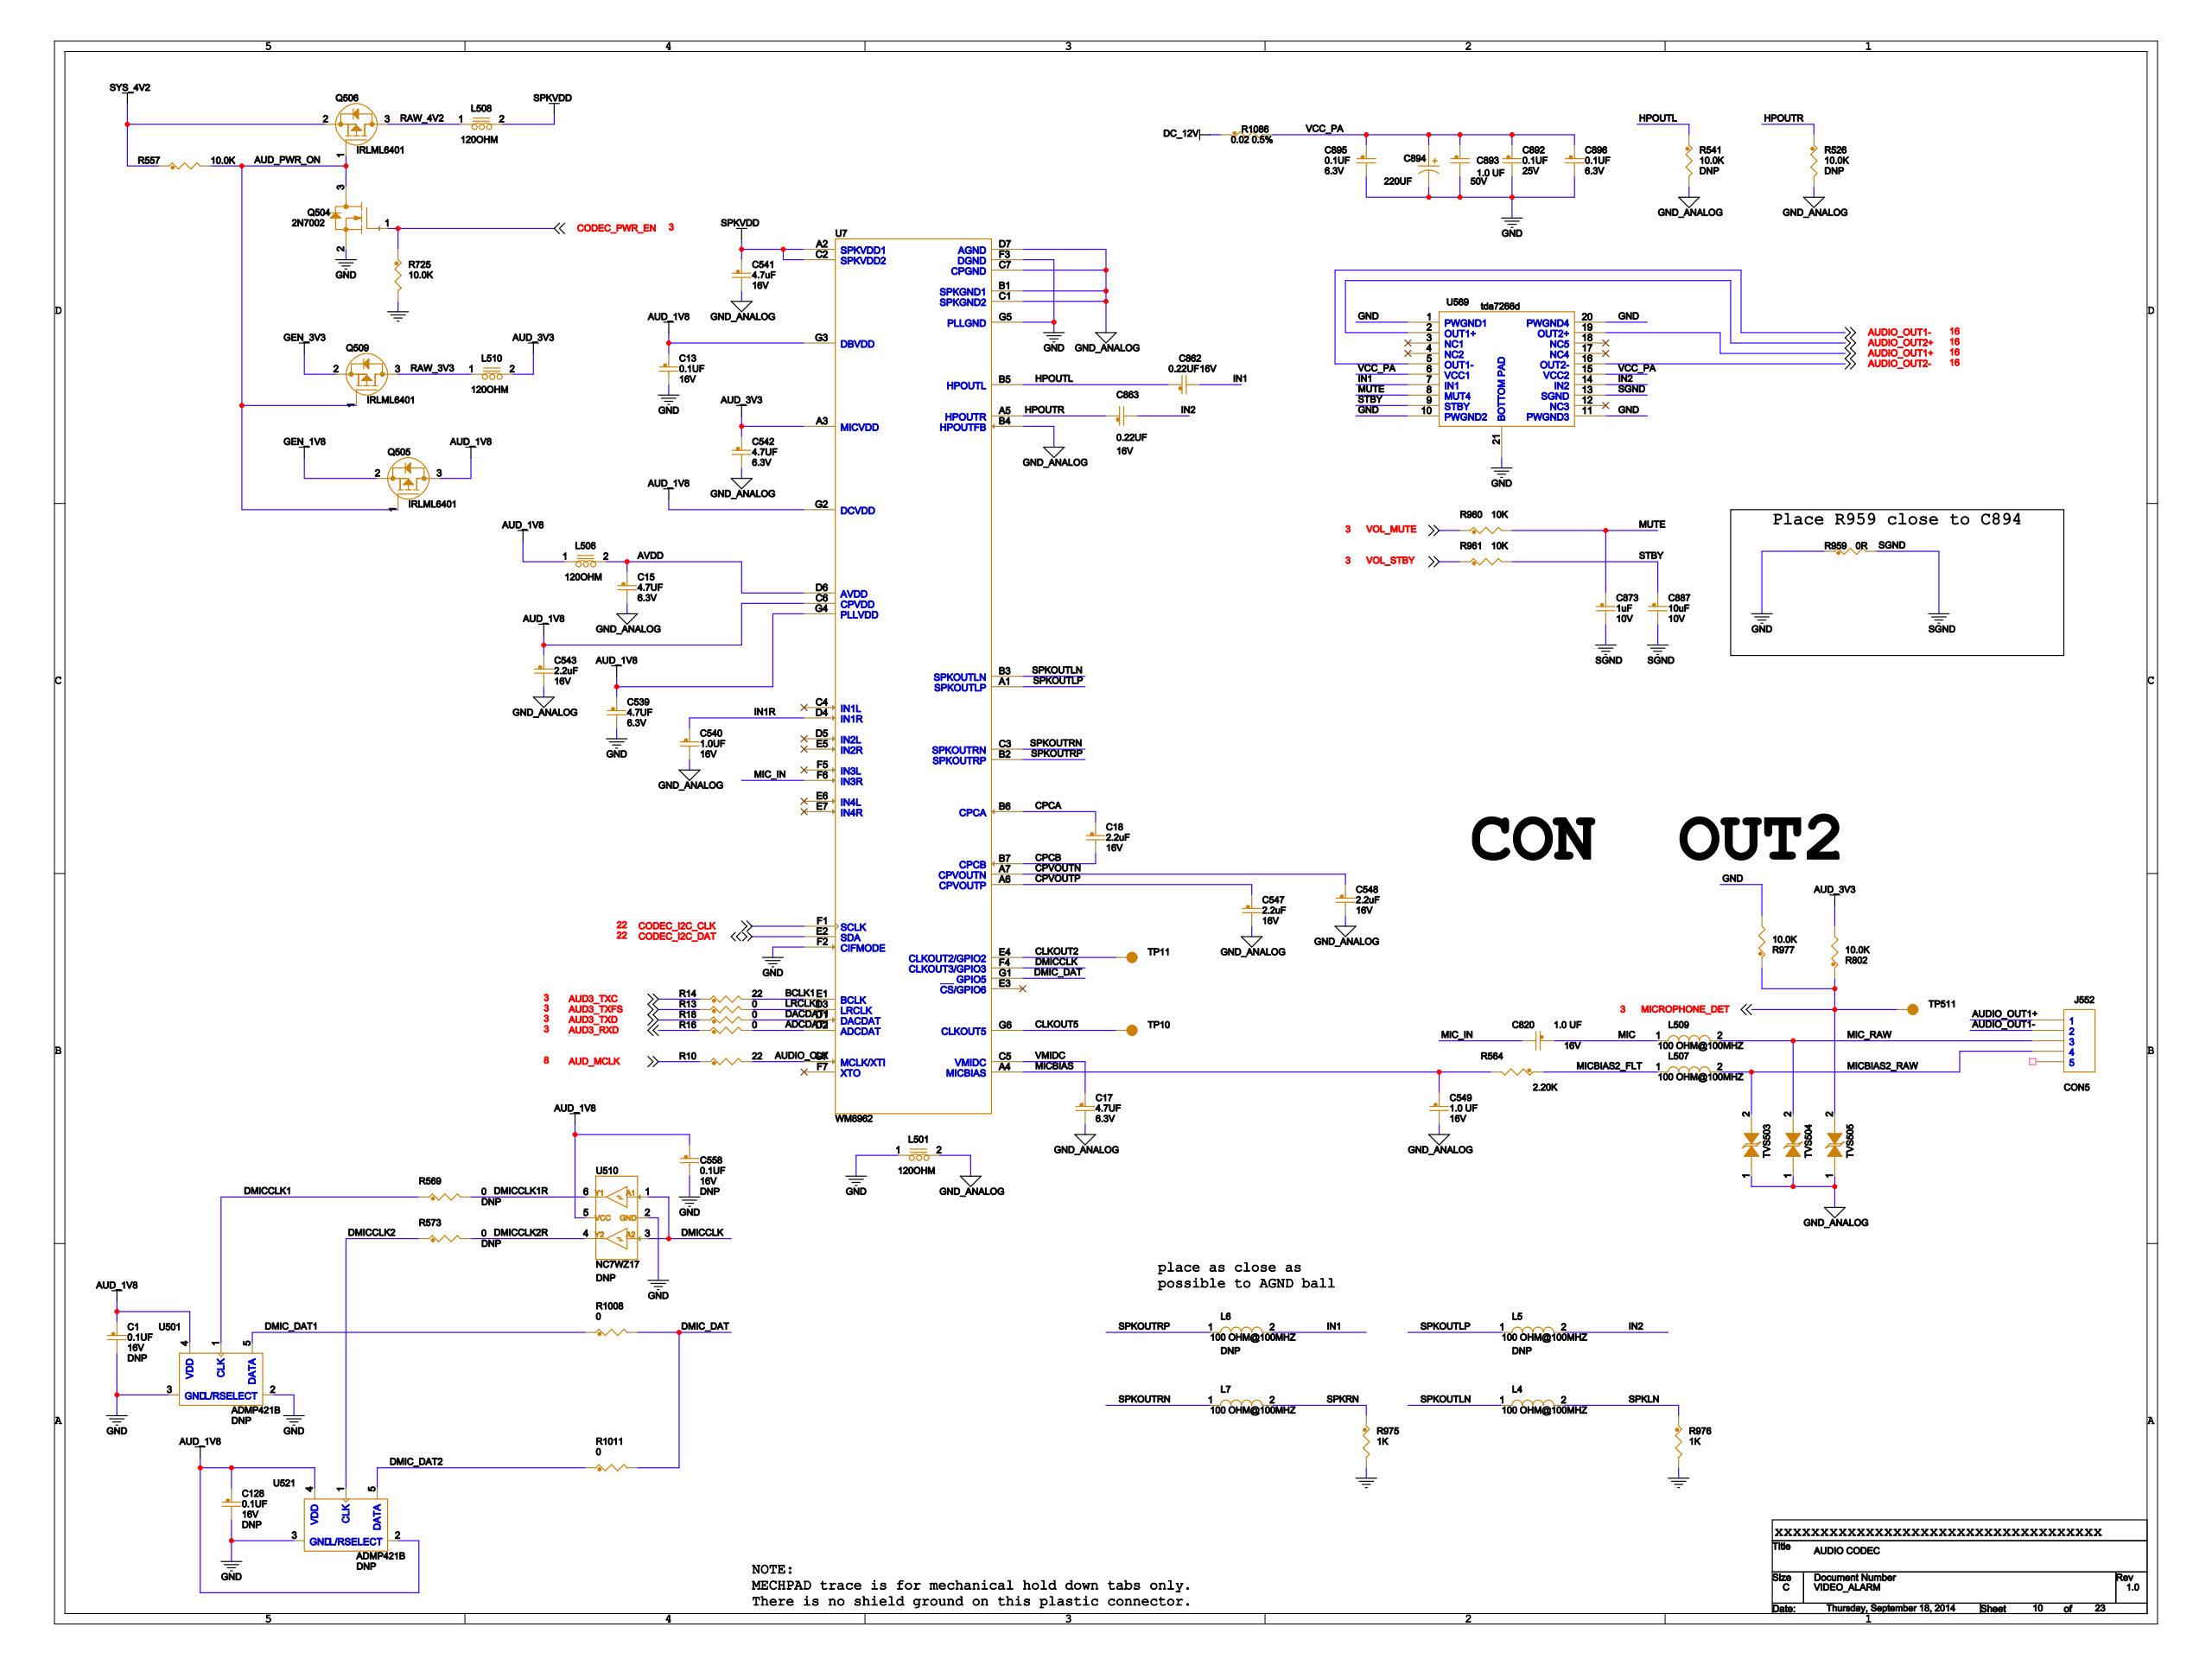Circuit board | Cadence Allegro | 994 parts | 728 nets | one sheet of the schematic
Parts on this sheet (reference | value | footprint):
C1 | 0.1UF | 0603_CC
C13 | 0.1UF | 0603_CC
C15 | 4.7UF | 0603_CC
C17 | 4.7UF | 0603_CC
C18 | 2.2uF | 0603_CC
C128 | 0.1UF | 0603_CC
C539 | 4.7UF | 0603_CC
C540 | 1.0UF | 0603_CC
C541 | 4.7uF | 0603_CC
C542 | 4.7UF | 0603_CC
C543 | 2.2uF | 0603_CC
C547 | 2.2uF | 0603_CC
C548 | 2.2uF | 0603_CC
C549 | 1.0 UF | 0603_CC
C558 | 0.1UF | 0603_CC
C820 | 1.0 UF | 0603_CC
C862 | 0.22UF | 0603_CC
C863 | 0.22UF | 0603_CC
C873 | 1uF | 0603_CC
C887 | 10uF | 0603_CC
C892 | 0.1UF | 0603_CC
C893 | 1.0 UF | 0603_CC
C894 | 220UF | CAPDIP0903
C895 | 0.1UF | 0603_CC
C896 | 0.1UF | 0603_CC
J552 | CON5 | CON5
L4 | 100 OHM@100MHZ | 0603_CC
L5 | 100 OHM@100MHZ | 0603_CC
L6 | 100 OHM@100MHZ | 0603_CC
L7 | 100 OHM@100MHZ | 0603_CC
L501 | 120OHM | 0603_CC
L506 | 120OHM | 0603_CC
L507 | 100 OHM@100MHZ | 0603_CC
L508 | 120OHM | 0603_CC
L509 | 100 OHM@100MHZ | 0603_CC
L510 | 120OHM | 0603_CC
Q504 | 2N7002 | SOT23
Q505 | IRLML6401 | SOT-23
Q506 | IRLML6401 | SOT-23
Q509 | IRLML6401 | SOT-23
R10 | 22 | 0603_CC
R13 | 0 | 0603_CC
R14 | 22 | 0603_CC
R16 | 0 | 0603_CC
R18 | 0 | 0603_CC
R526 | 10.0K | 0603_CC
R541 | 10.0K | 0603_CC
R557 | 10.0K | 0603_CC
R564 | 2.20K | 0603_CC
R569 | 0 | 0603_CC
R573 | 0 | 0603_CC
R725 | 10.0K | 0603_CC
R802 | 10.0K | 0603_CC
R959 | 0R | 0603_CC
R960 | 10K | 0603_CC
R961 | 10K | 0603_CC
R975 | 1K | 0603_CC
R976 | 1K | 0603_CC
R977 | 10.0K | 0603_CC
R1008 | 0 | 0805_CC
R1011 | 0 | 0805_CC
R1086 | 0.02 | 0805_CC
TP10 | TPAD_020 | TPAD_020
TP11 | TPAD_020 | TPAD_020
TP511 | TPAD_020 | TPAD_020
TVS503 | ESD9B3.3ST5G | SOD-923_NP
TVS504 | ESD9B3.3ST5G | SOD-923_NP
TVS505 | ESD9B3.3ST5G | SOD-923_NP
U7 | WM8962 | BGA49_0P5_3P62X4
U501 | ADMP421B | LGA5_CAV_4P1X3P1MM
U510 | NC7WZ17 | SC70_6LEAD
U521 | ADMP421B | LGA5_CAV_4P1X3P1MM
U569 | tda7266d | TDA7266D
Nets of these parts (net: part-pin ...):
GND: C1-2 C13-2 C128-2 C539-2 C558-2 C892-2 C893-2 C894-2 C895-2 C896-2 L501-1 Q504-2 R725-2 R959-1 R975-2 R976-2 R977-2 U501-2 U501-3 U510-2 U521-3 U569-1 U569-10 U569-11 U569-20 U569-21 U7-F2 U7-F3 U7-G5
GEN_3V3: Q509-2
SYS_4V2: Q506-2 R557-1
GEN_1V8: Q505-2
DC_12V: R1086-1
VCC_PA: C892-1 C893-1 C894-1 C895-1 C896-1 R1086-2 U569-6 U569-15
AUDIO_OUT1-: J552-2 U569-5
AUDIO_OUT1+: J552-1 U569-2
AUDIO_OUT2+: U569-19
AUDIO_OUT2-: U569-16
MICBIAS2_RAW: J552-4 L507-2 TVS503-2
MIC_RAW: J552-3 L509-2 TVS504-2
SGND: C873-2 C887-2 R959-2 U569-13
SPKLN: L4-2 R976-1
SPKRN: L7-2 R975-1
AUD_MCLK: R10-1
DMICCLK2: R573-1 U521-1
DMICCLK2R: R573-2 U510-4
DMICCLK1: R569-1 U501-1
DMICCLK1R: R569-2 U510-6
AUD3_TXD: R18-1
DACDAT1: R18-2 U7-D1
AUD3_RXD: R16-1
ADCDAT1: R16-2 U7-D2
AUD3_TXFS: R13-1
LRCLK1: R13-2 U7-D3
CODEC_I2C_CLK: U7-F1
CODEC_I2C_DAT: U7-E2
MICROPHONE_DET: R802-1 R977-1 TP511-1 TVS505-2
AUD_3V3: C542-1 L510-2 R802-2 U7-A3
CODEC_PWR_EN: Q504-1 R725-1
AUD_PWR_ON: Q504-3 Q505-1 Q506-1 Q509-1 R557-2
HPOUTL: C862-1 R541-1 U7-B5
GND_ANALOG: C15-2 C17-2 C540-2 C541-2 C542-2 C543-2 C547-2 C548-2 C549-2 L501-2 R526-2 R541-2 TVS503-1 TVS504-1 TVS505-1 U7-B1 U7-B4 U7-C1 U7-C7 U7-D7
HPOUTR: C863-1 R526-1 U7-A5
IN1R: C540-1 U7-D4
IN2: C863-2 L5-2 U569-14
IN1: C862-2 L6-2 U569-7
AUD_1V8: C1-1 C13-1 C128-1 C539-1 C543-1 C558-1 L506-1 Q505-3 U501-4 U510-5 U521-2 U521-4 U7-C6 U7-G2 U7-G3 U7-G4
AVDD: C15-1 L506-2 U7-D6
BCLK1: R14-2 U7-E1
CLKOUT2: TP11-1 U7-E4
DMICCLK: U510-1 U510-3 U7-F4
CLKOUT5: TP10-1 U7-G6
CPCA: C18-1 U7-B6
CPCB: C18-2 U7-B7
CPVOUTN: C548-1 U7-A7
CPVOUTP: C547-1 U7-A6
DMIC_DAT: R1008-2 R1011-2 U7-G1
MIC_IN: C820-2 U7-F6
AUDIO_CLK: R10-2 U7-G7
MICBIAS: C549-1 R564-2 U7-A4
SPKOUTLN: L4-1 U7-B3
SPKOUTLP: L5-1 U7-A1
SPKOUTRN: L7-1 U7-C3
SPKOUTRP: L6-1 U7-B2
SPKVDD: C541-1 L508-2 U7-A2 U7-C2
VMIDC: C17-1 U7-C5
MUTE: C873-1 R960-2 U569-8
STBY: C887-1 R961-2 U569-9
DMIC_DAT2: R1011-1 U521-5
DMIC_DAT1: R1008-1 U501-5
AUD3_TXC: R14-1
VOL_STBY: R961-1
VOL_MUTE: R960-1
MICBIAS2_FLT: L507-1 R564-1
RAW_3V3: L510-1 Q509-3
RAW_4V2: L508-1 Q506-3
MIC: C820-1 L509-1